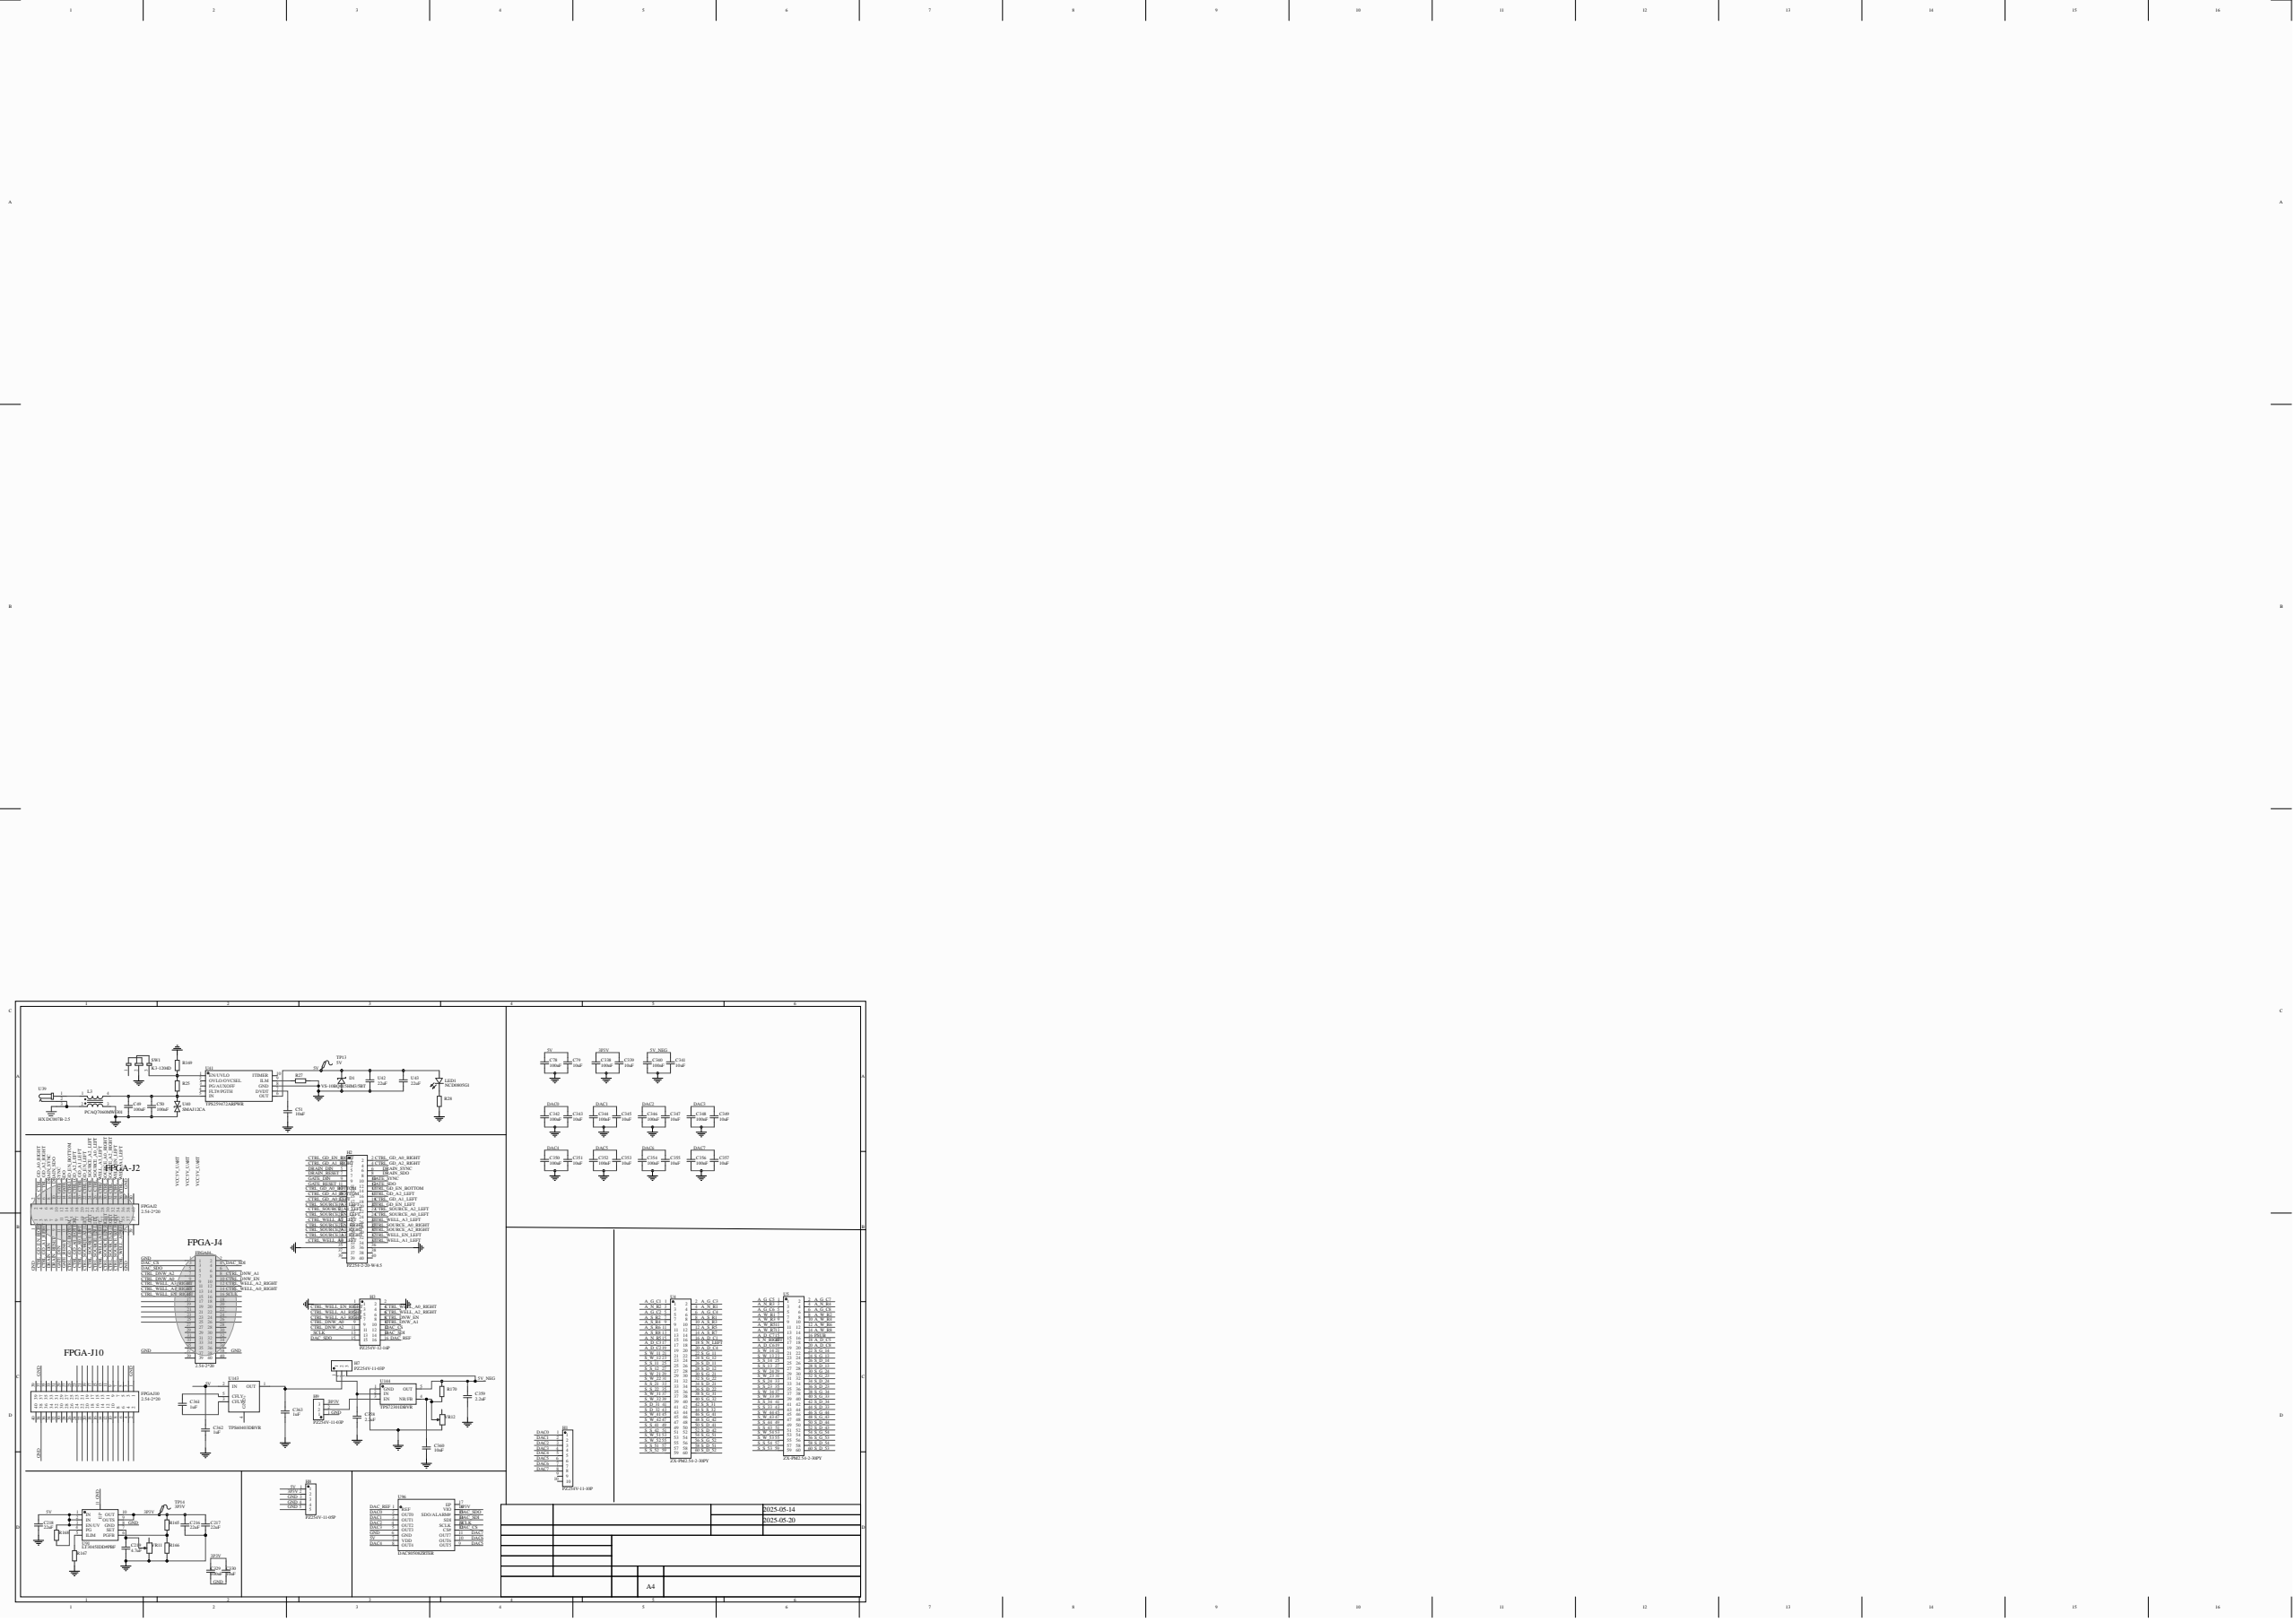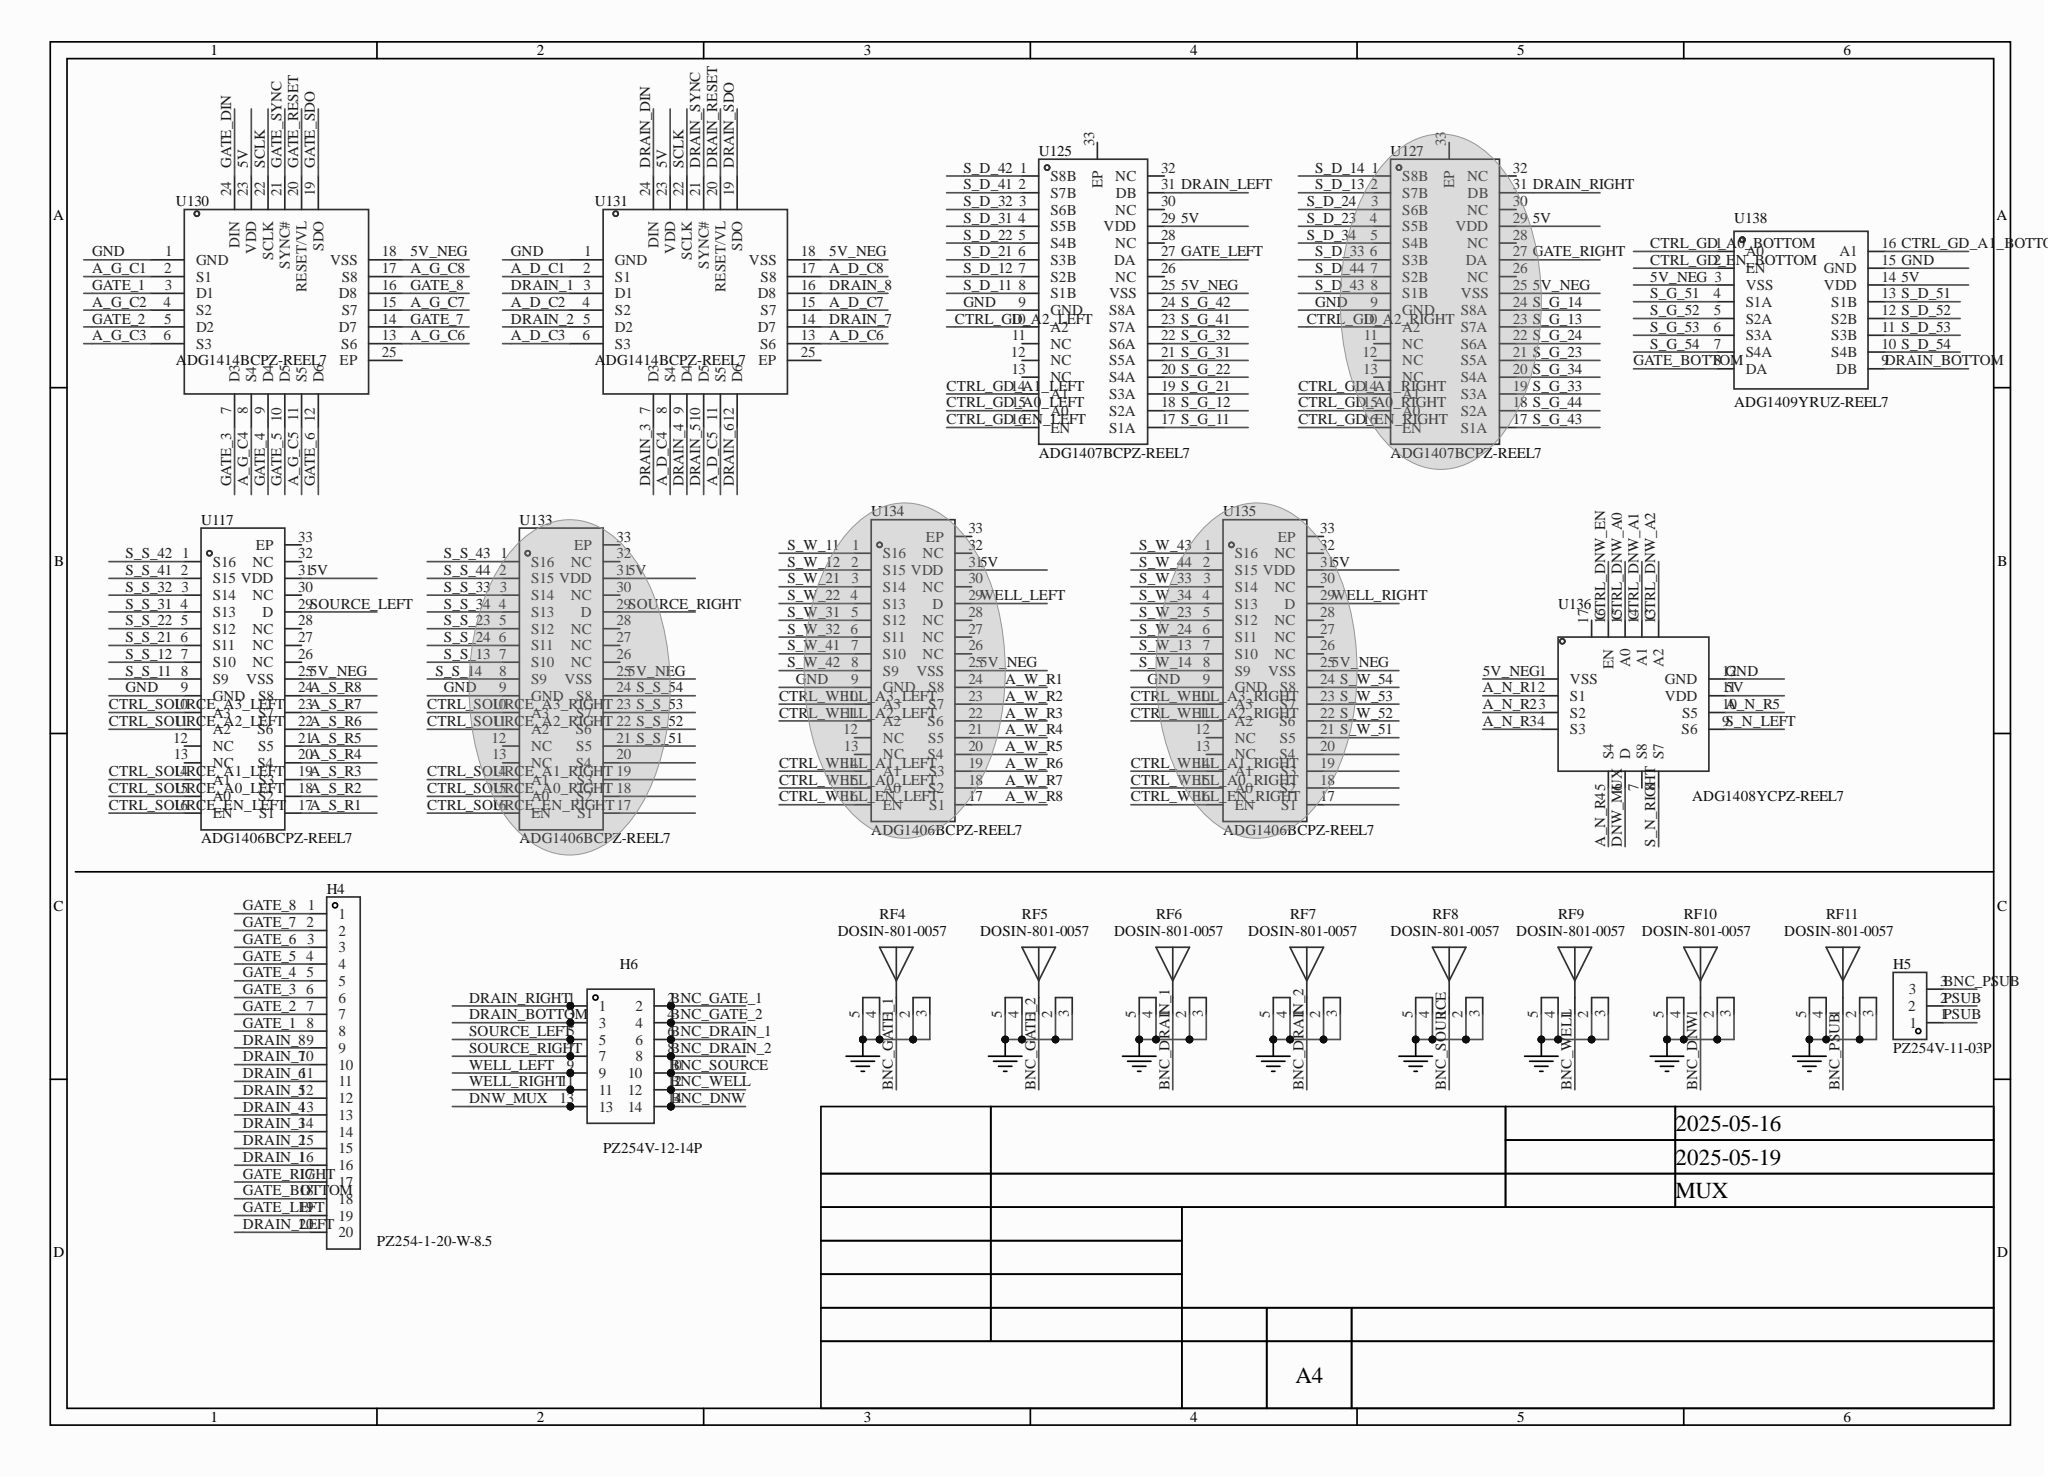Circuit board | Altium Designer | 95 parts | 232 nets
Bill of materials:
Comment,Description,Designator,Footprint,LibRef,Quantity
"100nF","","C49, C50, C78, C338, C340, C342, C344, C346, C348, C350, C352, C354, C356","C0603","CL10B104KA8NNNC, CL10B104JB8NNNC","13"
"10nF","","C51, C360","C0805","CL21B103KBANNNC","2"
"10uF","","C79, C339, C341, C343, C345, C347, C349, C351, C353, C355, C357","C0603","CL10A106KO8NQNC","11"
"22uF","","C216, C217, C218","C0603","CL10A226MO7JZNC","3"
"4.7uF","","C219","C0603","CL10A475KA8NQNC","1"
"100nF","","C329","C0805","CL21B104KCFNNNE","1"
"10uF","","C330","C0805","GRM21BR61H106KE43L","1"
"2.2uF","","C358, C359","C0603","CL10A225KB8NNNC","2"
"1uF","","C361, C362, C363","C0603","CL10A105KB8NNNC","3"
"VS-10BQ015HM3/5BT","","D1","SMB_L4.6-W3.6-LS5.3-RD","VS-10BQ015HM3/5BT","1"
"2.54-2*20","","FPGAJ2, FPGAJ4, FPGAJ10","HDR-TH_40P-P2.54-V-F-R2-C20-S2.54","2.54-2*20","3"
"PZ254V-11-10P","","H1","HDR-TH_10P-P2.54-V-M","PZ254V-11-10P","1"
"PZ254-2-20-W-8.5","","H2","HDR-TH_40P-P2.54-V-F-R2-C20-S2.54","PZ254-2-20-W-8.5_C2895000","1"
"PZ254V-12-16P","","H3","HDR-TH_16P-P2.54-V-M-R2-C8-S2.54","PZ254V-12-16P","1"
"PZ254-1-20-W-8.5","","H4","HDR-TH_20P-P2.54-V-M-1","PZ254-1-20-W-8.5","1"
"PZ254V-11-03P","","H5, H7, H9","HDR-TH_3P-P2.54-V-M","PZ254V-11-03P","3"
"PZ254V-12-14P","","H6","HDR-TH_14P-P2.54-V-M-R2-C7-S2.54","PZ254V-12-14P","1"
"PZ254V-11-05P","","H8","HDR-TH_5P-P2.54-V-M","PZ254V-11-05P","1"
"PCAQ7060MW-301","","L3","FILTER-SMD_4P-L7.0-W6.0-BL","PCAQ7060MW-301","1"
"NCD0805G1","","LED1","LED0805-R-RD","NCD0805G1","1"
"","","R25, R27, R28, R165, R166, R167, R168, R169, R170","R0603","0603WAF1004T5E, RT0603BRD07681RL, 0603WAF1001T5E, 0603WAF4533T5E, AR03BTC5002A, 0603WAF2490T5E, 0603WAF2003T5E, ERJ3RED3573V, 0603WAF7502T5E","9"
"DOSIN-801-0057","","RF4, RF5, RF6, RF7, RF8, RF9, RF10, RF11","ANT-TH_DOSIN-801-0057","DOSIN-801-0057","8"
"K3-1204D","","SW1","SW-TH_K3-1204D","K3-1204D","1"
"5V","","TP13","Test-Point-0.5mm","5V","1"
"3P3V","","TP14","Test-Point-0.5mm","3P3V","1"
"ZX-PM2.54-2-30PY","","U4, U5","HDR-TH_60P-P2.54-V-F-R2-C30-S2.54","ZX-PM2.54-2-30PY","2"
"HX DC007B-2.5","","U39","DC-IN-TH_HX-DC007B-2.5","HX DC007B-2.5","1"
"SMAJ12CA","","U40","SMA_L4.3-W2.7-LS5.1-BI","SMAJ12CA","1"
"TPS259472ARPWR","","U41","VQFN-10_L2.0-W2.0-P0.45-TL","TPS259472ARPWR","1"
"22uF","","U42, U43","C0805","CL21A226KOQNNNE","2"
"LT3045IDD#PBF","","U91","DFN-10_L3.0-W3.0-P0.50-BL-EP-3","LT3045IDD#PBF","1"
"DAC80508ZRTER","","U96","WQFN-16_L3.0-W3.0-P0.50-TL-EP0.8","DAC80508ZRTER","1"
"ADG1406BCPZ-REEL7","","U117, U133, U134, U135","LFCSP-32_L5.0-W5.0-P0.50-TL-EP3.1","ADG1406BCPZ-REEL7","4"
"ADG1407BCPZ-REEL7","","U125, U127","LFCSP-32_L5.0-W5.0-P0.50-BL-EP3.1","ADG1407BCPZ-REEL7","2"
"ADG1414BCPZ-REEL7","","U130, U131","LFCSP-24_L4.0-W4.0-P0.50-BL-EP","ADG1414BCPZ-REEL7","2"
"ADG1408YCPZ-REEL7","","U136","LFCSP-16_L4.0-W4.0-P0.65-BL-EP","ADG1408YCPZ-REEL7","1"
"ADG1409YRUZ-REEL7","","U138","TSSOP-16_L5.0-W4.4-P0.65-LS6.4-BL","ADG1409YRUZ-REEL7","1"
"TPS60403DBVR","","U143","SOT-23-5_L3.0-W1.7-P0.95-LS2.8-BR","TPS60403DBVR","1"
"TPS72301DBVR","","U144","SOT-23-5_L3.0-W1.7-P0.95-LS2.8-BR","TPS72301DBVR","1"
"","","VR11, VR12","RES-ADJ-SMD_3224W","3224W-1-503E","2"
Netlist (Protel format):
[
C49
C0603
100nF



]
[
C50
C0603
100nF



]
[
C51
C0805
10nF



]
[
C78
C0603
100nF



]
[
C79
C0603
10uF



]
[
C216
C0603
22uF



]
[
C217
C0603
22uF



]
[
C218
C0603
22uF



]
[
C219
C0603
4.7uF



]
[
C329
C0805
100nF



]
[
C330
C0805
10uF



]
[
C338
C0603
100nF



]
[
C339
C0603
10uF



]
[
C340
C0603
100nF



]
[
C341
C0603
10uF



]
[
C342
C0603
100nF



]
[
C343
C0603
10uF



]
[
C344
C0603
100nF



]
[
C345
C0603
10uF



]
[
C346
C0603
100nF



]
[
C347
C0603
10uF



]
[
C348
C0603
100nF



]
[
C349
C0603
10uF



]
[
C350
C0603
100nF



]
[
C351
C0603
10uF



]
[
C352
C0603
100nF



]
[
C353
C0603
10uF



]
[
C354
C0603
100nF



]
[
C355
C0603
10uF



]
[
C356
C0603
100nF



]
[
C357
C0603
10uF



]
[
C358
C0603
2.2uF



]
[
C359
C0603
2.2uF



]
[
C360
C0805
10nF



]
[
C361
C0603
1uF



]
[
C362
C0603
1uF



]
[
C363
C0603
1uF



]
[
D1
SMB_L4.6-W3.6-LS5.3-RD
VS-10BQ015HM3/5BT



]
[
FPGAJ2
HDR-TH_40P-P2.54-V-F-R2-C20-S2.54
2.54-2*20



]
[
FPGAJ4
HDR-TH_40P-P2.54-V-F-R2-C20-S2.54
2.54-2*20



]
[
FPGAJ10
HDR-TH_40P-P2.54-V-F-R2-C20-S2.54
2.54-2*20



]
[
H1
HDR-TH_10P-P2.54-V-M
PZ254V-11-10P



]
[
H2
HDR-TH_40P-P2.54-V-F-R2-C20-S2.54
PZ254-2-20-W-8.5



]
[
H3
HDR-TH_16P-P2.54-V-M-R2-C8-S2.54
PZ254V-12-16P



]
[
H4
HDR-TH_20P-P2.54-V-M-1
PZ254-1-20-W-8.5



]
[
H5
HDR-TH_3P-P2.54-V-M
PZ254V-11-03P



]
[
H6
HDR-TH_14P-P2.54-V-M-R2-C7-S2.54
PZ254V-12-14P



]
[
H7
HDR-TH_3P-P2.54-V-M
PZ254V-11-03P



]
[
H8
HDR-TH_5P-P2.54-V-M
PZ254V-11-05P



]
[
H9
HDR-TH_3P-P2.54-V-M
PZ254V-11-03P



]
[
L3
FILTER-SMD_4P-L7.0-W6.0-BL
PCAQ7060MW-301



]
[
LED1
LED0805-R-RD
NCD0805G1



]
[
R25
R0603




]
[
R27
R0603




]
[
R28
R0603




]
[
R165
R0603




]
[
R166
R0603




]
[
R167
R0603




]
[
R168
R0603




]
[
R169
R0603




]
[
R170
R0603




]
[
RF4
ANT-TH_DOSIN-801-0057
DOSIN-801-0057



]
[
RF5
ANT-TH_DOSIN-801-0057
DOSIN-801-0057



]
[
RF6
ANT-TH_DOSIN-801-0057
DOSIN-801-0057



]
[
RF7
ANT-TH_DOSIN-801-0057
DOSIN-801-0057



]
[
RF8
ANT-TH_DOSIN-801-0057
DOSIN-801-0057



]
[
RF9
ANT-TH_DOSIN-801-0057
DOSIN-801-0057



]
[
RF10
ANT-TH_DOSIN-801-0057
DOSIN-801-0057



]
[
RF11
ANT-TH_DOSIN-801-0057
DOSIN-801-0057



]
[
SW1
SW-TH_K3-1204D
K3-1204D



]
[
TP13
Test-Point-0.5mm
5V



]
[
TP14
Test-Point-0.5mm
3P3V



]
[
U4
HDR-TH_60P-P2.54-V-F-R2-C30-S2.54
ZX-PM2.54-2-30PY



]
[
U5
HDR-TH_60P-P2.54-V-F-R2-C30-S2.54
ZX-PM2.54-2-30PY



]
[
U39
DC-IN-TH_HX-DC007B-2.5
HX DC007B-2.5



]
[
U40
SMA_L4.3-W2.7-LS5.1-BI
SMAJ12CA



]
[
U41
VQFN-10_L2.0-W2.0-P0.45-TL
TPS259472ARPWR



]
[
U42
C0805
22uF



]
[
U43
C0805
22uF



]
[
U91
DFN-10_L3.0-W3.0-P0.50-BL-EP-3
LT3045IDD#PBF



]
[
U96
WQFN-16_L3.0-W3.0-P0.50-TL-EP0.8
DAC80508ZRTER



]
[
U117
LFCSP-32_L5.0-W5.0-P0.50-TL-EP3.1
ADG1406BCPZ-REEL7



]
[
U125
LFCSP-32_L5.0-W5.0-P0.50-BL-EP3.1
ADG1407BCPZ-REEL7



]
[
U127
LFCSP-32_L5.0-W5.0-P0.50-BL-EP3.1
ADG1407BCPZ-REEL7



]
[
U130
LFCSP-24_L4.0-W4.0-P0.50-BL-EP
ADG1414BCPZ-REEL7



]
[
U131
LFCSP-24_L4.0-W4.0-P0.50-BL-EP
ADG1414BCPZ-REEL7



]
[
U133
LFCSP-32_L5.0-W5.0-P0.50-TL-EP3.1
ADG1406BCPZ-REEL7



]
[
U134
LFCSP-32_L5.0-W5.0-P0.50-TL-EP3.1
ADG1406BCPZ-REEL7



]
[
U135
LFCSP-32_L5.0-W5.0-P0.50-TL-EP3.1
ADG1406BCPZ-REEL7



]
[
U136
LFCSP-16_L4.0-W4.0-P0.65-BL-EP
ADG1408YCPZ-REEL7



]
[
U138
TSSOP-16_L5.0-W4.4-P0.65-LS6.4-BL
ADG1409YRUZ-REEL7



]
[
U143
SOT-23-5_L3.0-W1.7-P0.95-LS2.8-BR
TPS60403DBVR



]
[
U144
SOT-23-5_L3.0-W1.7-P0.95-LS2.8-BR
TPS72301DBVR



]
[
VR11
RES-ADJ-SMD_3224W




]
[
VR12
RES-ADJ-SMD_3224W




]
(
WELL_RIGHT
H6-11
U135-29
)
(
WELL_LEFT
H6-9
U134-29
)
(
SOURCE_RIGHT
H6-7
U133-29
)
(
SOURCE_LEFT
H6-5
U117-29
)
(
SCLK
FPGAJ4-16
H3-13
U96-13
U130-22
U131-22
)
(
S_W_54
U5-53
U135-24
)
(
S_W_53
U5-55
U135-23
)
(
S_W_52
U4-55
U135-22
)
(
S_W_51
U4-53
U135-21
)
(
S_W_44
U5-45
U135-2
)
(
S_W_43
U5-47
U135-1
)
(
S_W_42
U4-47
U134-8
)
(
S_W_41
U4-45
U134-7
)
(
S_W_34
U5-37
U135-4
)
(
S_W_33
U5-39
U135-3
)
(
S_W_32
U4-39
U134-6
)
(
S_W_31
U4-37
U134-5
)
(
S_W_24
U5-29
U135-6
)
(
S_W_23
U5-31
U135-5
)
(
S_W_22
U4-31
U134-4
)
(
S_W_21
U4-29
U134-3
)
(
S_W_14
U5-21
U135-8
)
(
S_W_13
U5-23
U135-7
)
(
S_W_12
U4-23
U134-2
)
(
S_W_11
U4-21
U134-1
)
(
S_S_54
U5-57
U133-24
)
(
S_S_53
U5-59
U133-23
)
(
S_S_52
U4-59
U133-22
)
(
S_S_51
U4-57
U133-21
)
(
S_S_44
U5-49
U133-2
)
(
S_S_43
U5-51
U133-1
)
(
S_S_42
U4-51
U117-1
)
(
S_S_41
U4-49
U117-2
)
(
S_S_34
U5-41
U133-4
)
(
S_S_33
U5-43
U133-3
)
(
S_S_32
U4-44
U117-3
)
(
S_S_31
U4-42
U117-4
)
(
S_S_24
U5-33
U133-6
)
(
S_S_23
U5-35
U133-5
)
(
S_S_22
U4-35
U117-5
)
(
S_S_21
U4-33
U117-6
)
(
S_S_14
U5-25
U133-8
)
(
S_S_13
U5-27
U133-7
)
(
S_S_12
U4-27
U117-7
)
(
S_S_11
U4-25
U117-8
)
(
S_N_RIGHT
U5-17
U136-8
)
(
S_N_LEFT
U4-18
U136-9
)
(
S_G_54
U5-54
U138-7
)
(
S_G_53
U5-56
U138-6
)
(
S_G_52
U4-56
U138-5
)
(
S_G_51
U4-54
U138-4
)
(
S_G_44
U5-46
U127-18
)
(
S_G_43
U5-48
U127-17
)
(
S_G_42
U4-48
U125-24
)
(
S_G_41
U4-46
U125-23
)
(
S_G_34
U5-38
U127-20
)
(
S_G_33
U5-40
U127-19
)
(
S_G_32
U4-40
U125-22
)
(
S_G_31
U4-38
U125-21
)
(
S_G_24
U5-30
U127-22
)
(
S_G_23
U5-32
U127-21
)
(
S_G_22
U4-32
U125-20
)
(
S_G_21
U4-30
U125-19
)
(
S_G_14
U5-22
U127-24
)
(
S_G_13
U5-24
U127-23
)
(
S_G_12
U4-24
U125-18
)
(
S_G_11
U4-22
U125-17
)
(
S_D_54
U5-58
U138-10
)
(
S_D_53
U5-60
U138-11
)
(
S_D_52
U4-60
U138-12
)
(
S_D_51
U4-58
U138-13
)
(
S_D_44
U5-50
U127-7
)
(
S_D_43
U5-52
U127-8
)
(
S_D_42
U4-52
U125-1
)
(
S_D_41
U4-50
U125-2
)
(
S_D_34
U5-42
U127-5
)
(
S_D_33
U5-44
U127-6
)
(
S_D_32
U4-43
U125-3
)
(
S_D_31
U4-41
U125-4
)
(
S_D_24
U5-34
U127-3
)
(
S_D_23
U5-36
U127-4
)
(
S_D_22
U4-36
U125-5
)
(
S_D_21
U4-34
U125-6
)
(
S_D_14
U5-26
U127-1
)
(
S_D_13
U5-28
U127-2
)
(
S_D_12
U4-28
U125-7
)
(
S_D_11
U4-26
U125-8
)
(
PSUB
H5-1
H5-2
U5-16
)
(
NetR168_1
R168-1
U91-4
)
(
NetR167_2
R167-2
U91-5
)
(
NetR165_1
R165-1
R166-2
U91-6
)
(
NetR27_1
R27-1
U41-9
)
(
NetR25_2
R25-2
R169-1
SW1-3
U41-1
)
(
NetLED1_2
LED1-2
R28-2
)
(
NetL3_2
L3-2
U39-2
U39-3
)
(
NetL3_1
L3-1
U39-1
)
(
NetH9_2
H9-2
U144-3
)
(
NetC363_2
C363-2
H7-2
U143-1
)
(
NetC361_2
C361-2
U143-5
)
(
NetC361_1
C361-1
U143-3
)
(
NetC360_2
C360-2
R170-1
U144-4
VR12-2
)
(
NetC358_2
C358-2
H7-1
U144-2
)
(
NetC219_2
C219-2
U91-7
VR11-2
)
(
NetC51_2
C51-2
U41-7
)
(
NetC49_2
C49-2
C50-2
L3-4
R25-1
U40-2
U41-5
)
(
GND
C49-1
C50-1
C51-1
C78-1
C79-1
C216-1
C217-1
C218-1
C219-1
C329-1
C330-1
C338-1
C339-1
C340-1
C341-1
C342-1
C343-1
C344-1
C345-1
C346-1
C347-1
C348-1
C349-1
C350-1
C351-1
C352-1
C353-1
C354-1
C355-1
C356-1
C357-1
C358-1
C359-1
C360-1
C362-1
C363-1
D1-2
FPGAJ2-1
FPGAJ2-37
FPGAJ2-38
FPGAJ4-1
FPGAJ4-37
FPGAJ4-38
FPGAJ10-1
FPGAJ10-37
FPGAJ10-38
H2-35
H2-36
H3-1
H3-2
H8-3
H8-4
H8-5
H9-1
L3-3
R27-2
R28-1
R166-1
R167-1
R169-2
RF4-2
RF4-3
RF4-4
RF4-5
RF5-2
RF5-3
RF5-4
RF5-5
RF6-2
RF6-3
RF6-4
RF6-5
RF7-2
RF7-3
RF7-4
RF7-5
RF8-2
RF8-3
RF8-4
RF8-5
RF9-2
RF9-3
RF9-4
RF9-5
RF10-2
RF10-3
RF10-4
RF10-5
RF11-2
RF11-3
RF11-4
RF11-5
SW1-2
U40-1
U41-8
U42-1
U43-1
U91-8
U91-11
U96-6
U117-9
U125-9
U127-9
U130-1
U131-1
U133-9
U134-9
U135-9
U136-12
U138-15
U144-1
VR11-3
VR12-3
)
(
GATE_SYNC
FPGAJ2-12
H2-10
U130-21
)
(
GATE_SDO
FPGAJ2-14
H2-12
U130-19
)
(
GATE_RIGHT
H4-17
U127-27
)
(
GATE_RESET
FPGAJ2-13
H2-11
U130-20
)
(
GATE_LEFT
H4-19
U125-27
)
(
GATE_DIN
FPGAJ2-11
H2-9
U130-24
)
(
GATE_BOTTOM
H4-18
U138-8
)
(
GATE_8
H4-1
U130-16
)
(
GATE_7
H4-2
U130-14
)
(
GATE_6
H4-3
U130-12
)
(
GATE_5
H4-4
U130-10
)
(
GATE_4
H4-5
U130-9
)
(
GATE_3
H4-6
U130-7
)
(
GATE_2
H4-7
U130-5
)
(
GATE_1
H4-8
U130-3
)
(
DRAIN_SYNC
FPGAJ2-8
H2-6
U131-21
)
(
DRAIN_SDO
FPGAJ2-10
H2-8
U131-19
)
(
DRAIN_RIGHT
H6-1
U127-31
)
(
DRAIN_RESET
FPGAJ2-9
H2-7
U131-20
)
(
DRAIN_LEFT
H4-20
U125-31
)
(
DRAIN_DIN
FPGAJ2-7
H2-5
U131-24
)
(
DRAIN_BOTTOM
H6-3
U138-9
)
(
DRAIN_8
H4-9
U131-16
)
(
DRAIN_7
H4-10
U131-14
)
(
DRAIN_6
H4-11
U131-12
)
(
DRAIN_5
H4-12
U131-10
)
(
DRAIN_4
H4-13
U131-9
)
(
DRAIN_3
H4-14
U131-7
)
(
DRAIN_2
H4-15
U131-5
)
(
DRAIN_1
H4-16
U131-3
)
(
DNW_MUX
H6-13
U136-6
)
(
DAC_SDO
FPGAJ4-5
H3-15
U96-15
)
(
DAC_SDI
FPGAJ4-4
H3-14
U96-14
)
(
DAC_REF
H3-16
U96-1
)
(
DAC_CS
FPGAJ4-3
H3-12
U96-12
)
(
DAC7
C356-2
C357-2
H1-8
U96-11
)
(
DAC6
C354-2
C355-2
H1-7
U96-10
)
(
DAC5
C352-2
C353-2
H1-6
U96-9
)
(
DAC4
C350-2
C351-2
H1-5
U96-8
)
(
DAC3
C348-2
C349-2
H1-4
U96-5
)
(
DAC2
C346-2
C347-2
H1-3
U96-4
)
(
DAC1
C344-2
C345-2
H1-2
U96-3
)
(
DAC0
C342-2
C343-2
H1-1
U96-2
)
(
CTRL_WELL_EN_RIGHT
FPGAJ4-15
H3-3
U135-16
)
(
CTRL_WELL_EN_LEFT
FPGAJ2-34
H2-32
U134-16
)
(
CTRL_WELL_A3_RIGHT
FPGAJ4-11
H3-7
U135-10
)
(
CTRL_WELL_A3_LEFT
FPGAJ2-28
H2-26
U134-10
)
(
CTRL_WELL_A2_RIGHT
FPGAJ4-12
H3-6
U135-11
)
(
CTRL_WELL_A2_LEFT
FPGAJ2-27
H2-25
U134-11
)
(
CTRL_WELL_A1_RIGHT
FPGAJ4-13
H3-5
U135-14
)
(
CTRL_WELL_A1_LEFT
FPGAJ2-36
H2-34
U134-14
)
(
CTRL_WELL_A0_RIGHT
FPGAJ4-14
H3-4
U135-15
)
(
CTRL_WELL_A0_LEFT
FPGAJ2-35
H2-33
U134-15
)
(
CTRL_SOURCE_EN_RIGHT
FPGAJ2-29
H2-27
U133-16
)
(
CTRL_SOURCE_EN_LEFT
FPGAJ2-25
H2-23
U117-16
)
(
CTRL_SOURCE_A3_RIGHT
FPGAJ2-33
H2-31
U133-10
)
(
CTRL_SOURCE_A3_LEFT
FPGAJ2-21
H2-19
U117-10
)
(
CTRL_SOURCE_A2_RIGHT
FPGAJ2-32
H2-30
U133-11
)
(
CTRL_SOURCE_A2_LEFT
FPGAJ2-24
H2-22
U117-11
)
(
CTRL_SOURCE_A1_RIGHT
FPGAJ2-31
H2-29
U133-14
)
(
CTRL_SOURCE_A1_LEFT
FPGAJ2-23
H2-21
U117-14
)
(
CTRL_SOURCE_A0_RIGHT
FPGAJ2-30
H2-28
U133-15
)
(
CTRL_SOURCE_A0_LEFT
FPGAJ2-26
H2-24
U117-15
)
(
CTRL_GD_EN_RIGHT
FPGAJ2-3
H2-1
U127-16
)
(
CTRL_GD_EN_LEFT
FPGAJ2-22
H2-20
U125-16
)
(
CTRL_GD_EN_BOTTOM
FPGAJ2-16
H2-14
U138-2
)
(
CTRL_GD_A2_RIGHT
FPGAJ2-6
H2-4
U127-10
)
(
CTRL_GD_A2_LEFT
FPGAJ2-18
H2-16
U125-10
)
(
CTRL_GD_A1_RIGHT
FPGAJ2-5
H2-3
U127-14
)
(
CTRL_GD_A1_LEFT
FPGAJ2-20
H2-18
U125-14
)
(
CTRL_GD_A1_BOTTOM
FPGAJ2-17
H2-15
U138-16
)
(
CTRL_GD_A0_RIGHT
FPGAJ2-4
H2-2
U127-15
)
(
CTRL_GD_A0_LEFT
FPGAJ2-19
H2-17
U125-15
)
(
CTRL_GD_A0_BOTTOM
FPGAJ2-15
H2-13
U138-1
)
(
CTRL_DNW_EN
FPGAJ4-10
H3-8
U136-16
)
(
CTRL_DNW_A2
FPGAJ4-7
H3-11
U136-13
)
(
CTRL_DNW_A1
FPGAJ4-8
H3-10
U136-14
)
(
CTRL_DNW_A0
FPGAJ4-9
H3-9
U136-15
)
(
BNC_WELL
H6-12
RF9-1
)
(
BNC_SOURCE
H6-10
RF8-1
)
(
BNC_PSUB
H5-3
RF11-1
)
(
BNC_GATE_2
H6-4
RF5-1
)
(
BNC_GATE_1
H6-2
RF4-1
)
(
BNC_DRAIN_2
H6-8
RF7-1
)
(
BNC_DRAIN_1
H6-6
RF6-1
)
(
BNC_DNW
H6-14
RF10-1
)
(
A_W_R8
U5-14
U134-17
)
(
A_W_R7
U5-13
U134-18
)
(
A_W_R6
U5-12
U134-19
)
(
A_W_R5
U5-11
U134-20
)
(
A_W_R4
U5-10
U134-21
)
(
A_W_R3
U5-9
U134-22
)
(
A_W_R2
U5-8
U134-23
)
(
A_W_R1
U5-7
U134-24
)
(
A_S_R8
U4-13
U117-24
)
(
A_S_R7
U4-14
U117-23
)
(
A_S_R6
U4-11
U117-22
)
(
A_S_R5
U4-12
U117-21
)
(
A_S_R4
U4-9
U117-20
)
(
A_S_R3
U4-10
U117-19
)
(
A_S_R2
U4-7
U117-18
)
(
A_S_R1
U4-8
U117-17
)
(
A_N_R5
U4-15
U136-10
)
(
A_N_R4
U5-4
U136-5
)
(
A_N_R3
U5-3
U136-4
)
(
A_N_R2
U4-3
U136-3
)
(
A_N_R1
U4-4
U136-2
)
(
A_G_C8
U5-6
U130-17
)
(
A_G_C7
U5-2
U130-15
)
(
A_G_C6
U5-5
U130-13
)
(
A_G_C5
U5-1
U130-11
)
(
A_G_C4
U4-6
U130-8
)
(
A_G_C3
U4-2
U130-6
)
(
A_G_C2
U4-5
U130-4
)
(
A_G_C1
U4-1
U130-2
)
(
A_D_C8
U5-20
U131-17
)
(
A_D_C7
U5-15
U131-15
)
(
A_D_C6
U5-19
U131-13
)
(
A_D_C5
U5-18
U131-11
)
(
A_D_C4
U4-20
U131-8
)
(
A_D_C3
U4-17
U131-6
)
(
A_D_C2
U4-19
U131-4
)
(
A_D_C1
U4-16
U131-2
)
(
5V_NEG
C340-2
C341-2
C359-2
H7-3
R170-2
U117-25
U125-25
U127-25
U130-18
U131-18
U133-25
U134-25
U135-25
U136-1
U138-3
U144-5
)
(
5V
C78-2
C79-2
C218-2
C362-2
D1-1
H8-1
LED1-1
R168-2
TP13-1
U41-6
U42-2
U43-2
U91-1
U91-2
U91-3
U96-7
U117-31
U125-29
U127-29
U130-23
U131-23
U133-31
U134-31
U135-31
U136-11
U138-14
U143-2
)
(
3P3V
C216-2
C217-2
C329-2
C330-2
C338-2
C339-2
H8-2
H9-3
R165-2
TP14-1
U91-9
U91-10
U96-16
)